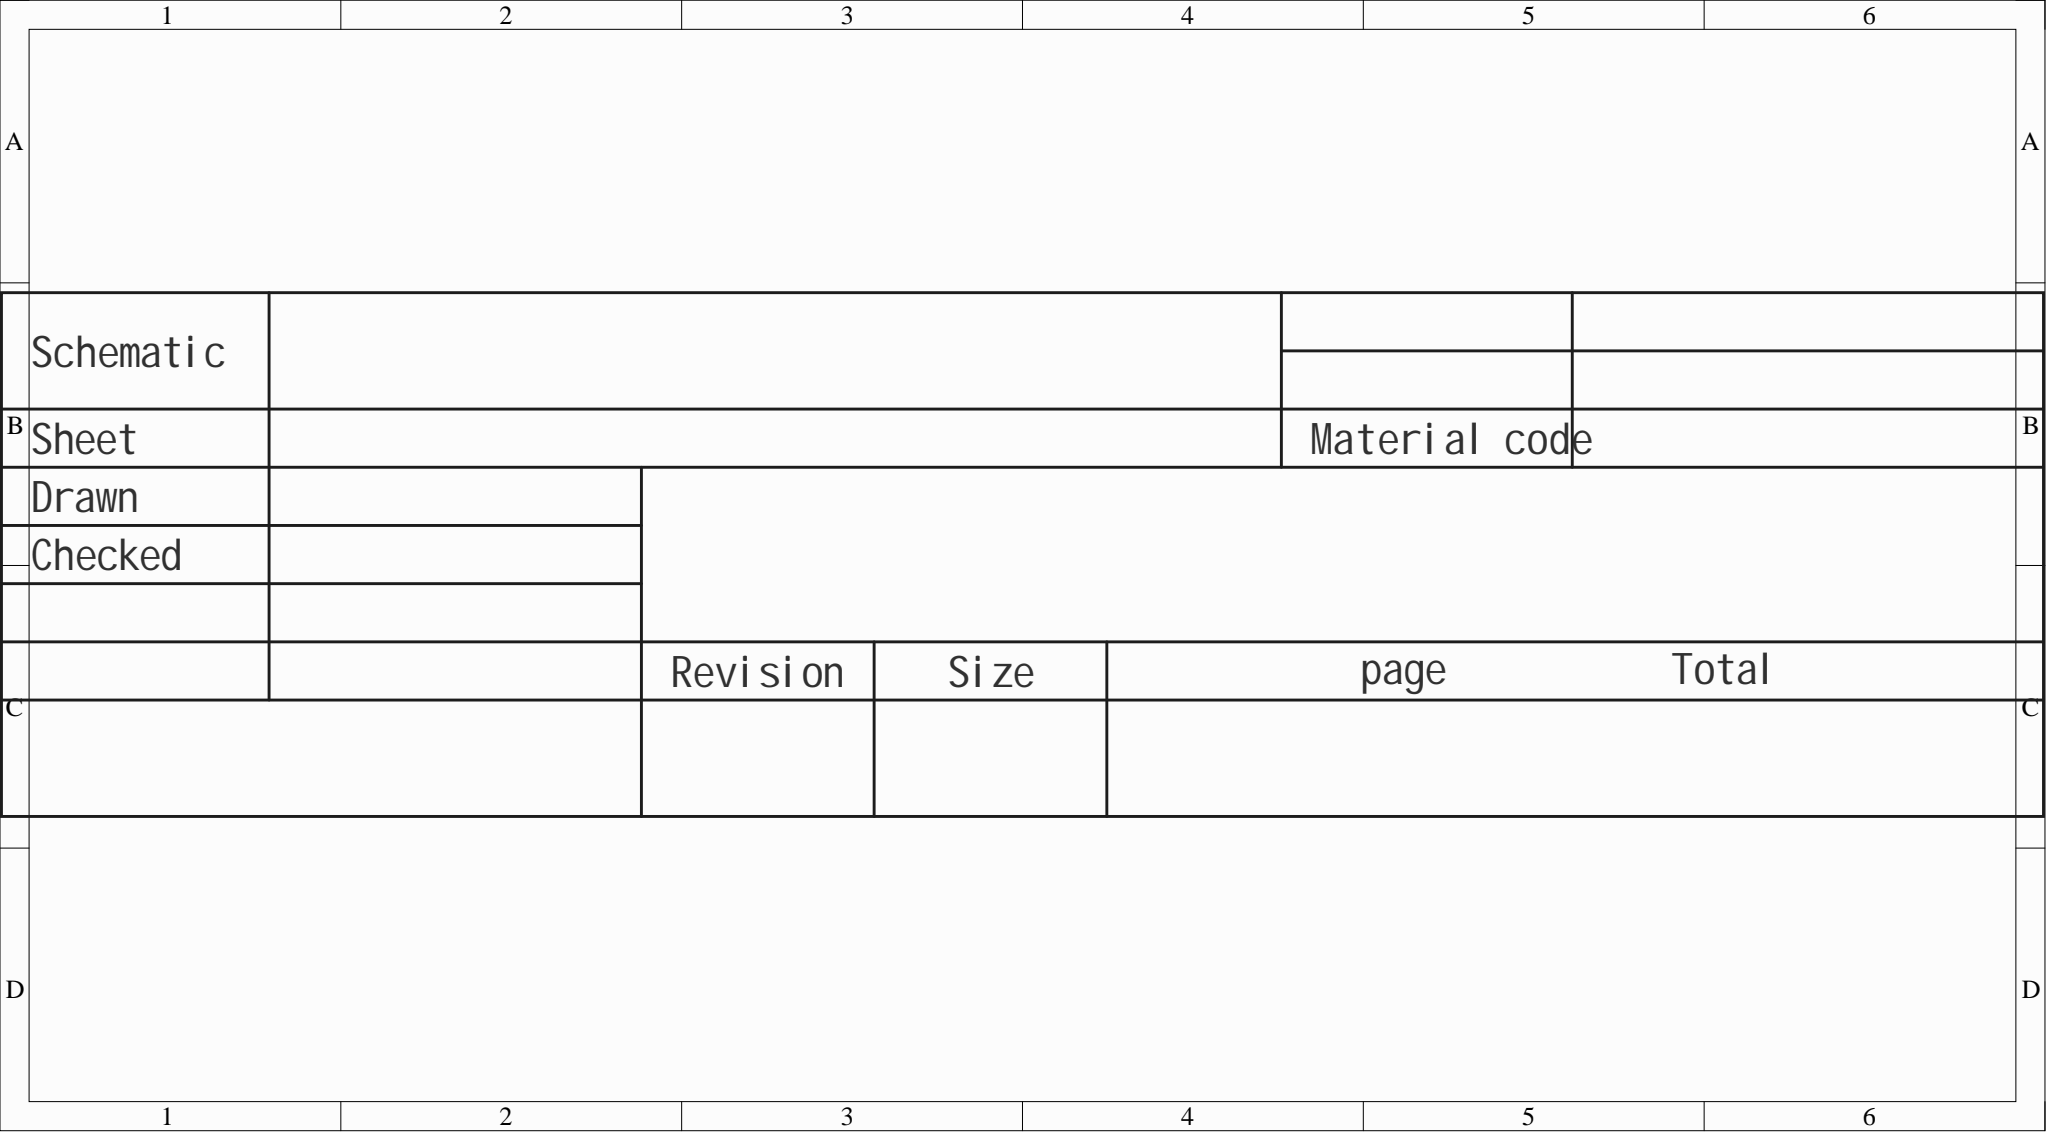Circuit board | Altium Designer | 63 parts | 46 nets
Bill of materials:
Comment,Description,Designator,Footprint,LibRef,Quantity
"100uF","","C1, C2","CAP-TH_BD8.0-P3.50-D0.6-FD_1","100uF","2"
"22uF","Capacitance:22uF;Accuracy:±10%;Rated voltage:16V;ESR:2Ω@100kHz;","C3, C8","CAP-TH_BD5.0-P2.5-D0.5-FD","TAP226K016SCS","2"
"100nF","","C4, C6, C9","CAP-TH_L5.0-W2.5-P5.00-D1.0","100nF","3"
"100UF","Capacitance:100nF;Rated voltage:50V;Ripple current:1A@100kHz;ESR:-;","C5","CAP-TH_BD5.0-P2.00-D0.8-FD","0.1uF 50V 5*11","1"
"4.7uF","Capacitance:4.7uF;Accuracy:±20%;Rated voltage:400V;Ripple current:140mA@100kHz;ESR:23.5Ω@100kHz;","C7","CAP-TH_BD6.3-P2.50-D1.0-FD","LKMC1202G4R7MF","1"
"","","D1","DO_1N4007","D_1N4007A","1"
"","","D2, D3","LED-TH_5mm","LED_TH-R_5mm, LED_TH-G_5mm","2"
"","","H1, H2, H3","HDR-TH_5P-P2.54-V-M","HDR-M_2.54_1x5P","3"
"38K infrared receiver, side-mounted","","OPTO1","OPTO-TH_3P-BD5.9-P2.54","红外38K接收管-侧放","1"
"9013G","","Q1, Q2, Q3, Q4, Q5, Q6, Q7, Q8, Q9, Q10, Q11, Q12, Q13","TO-92-3_L4.9-W3.7-P1.27-L","9013G","13"
"10kΩ","","R1, R7, R13, R15, R18","Res_1/4W","Res_AXIAL-1/4W","5"
"68kΩ","","R2","Res_1/4W","Res_AXIAL-1/4W","1"
"20kΩ","","R3, R23, R25, R30","Res_1/4W","Res_AXIAL-1/4W","4"
"680kΩ","","R4","Res_1/4W","Res_AXIAL-1/4W","1"
"27kΩ","","R5, R24, R28","Res_1/4W","Res_AXIAL-1/4W","3"
"5.1kΩ","","R6, R9, R12, R17, R22","Res_1/4W","Res_AXIAL-1/4W","5"
"51kΩ","","R8, R10, R11, R14, R16, R19, R20","Res_1/4W","Res_AXIAL-1/4W","7"
"100Ω","","R21","Res_1/4W","Res_AXIAL-1/4W","1"
"2kΩ","","R26, R27","Res_1/4W","Res_AXIAL-1/4W","2"
"300Ω","","R29","Res_1/4W","Res_AXIAL-1/4W","1"
"L7805","Fixed output; positive polarity; max input voltage 35V; output voltage 5V; output current 1.2A; ripple rejection (PSRR) 62dB@(120Hz)","U1","TO-220AB-3_L10.4-W4.6-P2.54-L","L7805","1"
"NE555","Single-precision timer 8-PDIP 0 to 70","U2, U4","PDIP-8_L9.6-W6.4-P2.54-LS7.9-BL-1","NE555PE4","2"
"","","U5","DIP-8_L9.9-W6.4-P2.54-LS7.6-BL","语音模块sop-8","1"
Netlist (Protel format):
[
C1
CAP-TH_BD8.0-P3.50-D0.6-FD_1
100uF



]
[
C2
CAP-TH_BD8.0-P3.50-D0.6-FD_1
100uF



]
[
C3
CAP-TH_BD5.0-P2.5-D0.5-FD
22uF



]
[
C4
CAP-TH_L5.0-W2.5-P5.00-D1.0
100nF



]
[
C5
CAP-TH_BD5.0-P2.00-D0.8-FD
100UF



]
[
C6
CAP-TH_L5.0-W2.5-P5.00-D1.0
100nF



]
[
C7
CAP-TH_BD6.3-P2.50-D1.0-FD
4.7uF



]
[
C8
CAP-TH_BD5.0-P2.5-D0.5-FD
22uF



]
[
C9
CAP-TH_L5.0-W2.5-P5.00-D1.0
100nF



]
[
D1
DO_1N4007




]
[
D2
LED-TH_5mm




]
[
D3
LED-TH_5mm




]
[
H1
HDR-TH_5P-P2.54-V-M




]
[
H2
HDR-TH_5P-P2.54-V-M




]
[
H3
HDR-TH_5P-P2.54-V-M




]
[
OPTO1
OPTO-TH_3P-BD5.9-P2.54
38K infrared receiver, side-mounted



]
[
Q1
TO-92-3_L4.9-W3.7-P1.27-L
9013G



]
[
Q2
TO-92-3_L4.9-W3.7-P1.27-L
9013G



]
[
Q3
TO-92-3_L4.9-W3.7-P1.27-L
9013G



]
[
Q4
TO-92-3_L4.9-W3.7-P1.27-L
9013G



]
[
Q5
TO-92-3_L4.9-W3.7-P1.27-L
9013G



]
[
Q6
TO-92-3_L4.9-W3.7-P1.27-L
9013G



]
[
Q7
TO-92-3_L4.9-W3.7-P1.27-L
9013G



]
[
Q8
TO-92-3_L4.9-W3.7-P1.27-L
9013G



]
[
Q9
TO-92-3_L4.9-W3.7-P1.27-L
9013G



]
[
Q10
TO-92-3_L4.9-W3.7-P1.27-L
9013G



]
[
Q11
TO-92-3_L4.9-W3.7-P1.27-L
9013G



]
[
Q12
TO-92-3_L4.9-W3.7-P1.27-L
9013G



]
[
Q13
TO-92-3_L4.9-W3.7-P1.27-L
9013G



]
[
R1
Res_1/4W
10kΩ



]
[
R2
Res_1/4W
68kΩ



]
[
R3
Res_1/4W
20kΩ



]
[
R4
Res_1/4W
680kΩ



]
[
R5
Res_1/4W
27kΩ



]
[
R6
Res_1/4W
5.1kΩ



]
[
R7
Res_1/4W
10kΩ



]
[
R8
Res_1/4W
51kΩ



]
[
R9
Res_1/4W
5.1kΩ



]
[
R10
Res_1/4W
51kΩ



]
[
R11
Res_1/4W
51kΩ



]
[
R12
Res_1/4W
5.1kΩ



]
[
R13
Res_1/4W
10kΩ



]
[
R14
Res_1/4W
51kΩ



]
[
R15
Res_1/4W
10kΩ



]
[
R16
Res_1/4W
51kΩ



]
[
R17
Res_1/4W
5.1kΩ



]
[
R18
Res_1/4W
10kΩ



]
[
R19
Res_1/4W
51kΩ



]
[
R20
Res_1/4W
51kΩ



]
[
R21
Res_1/4W
100Ω



]
[
R22
Res_1/4W
5.1kΩ



]
[
R23
Res_1/4W
20kΩ



]
[
R24
Res_1/4W
27kΩ



]
[
R25
Res_1/4W
20kΩ



]
[
R26
Res_1/4W
2kΩ



]
[
R27
Res_1/4W
2kΩ



]
[
R28
Res_1/4W
27kΩ



]
[
R29
Res_1/4W
300Ω



]
[
R30
Res_1/4W
20kΩ



]
[
U1
TO-220AB-3_L10.4-W4.6-P2.54-L
L7805



]
[
U2
PDIP-8_L9.6-W6.4-P2.54-LS7.9-BL-1
NE555



]
[
U4
PDIP-8_L9.6-W6.4-P2.54-LS7.9-BL-1
NE555



]
[
U5
DIP-8_L9.9-W6.4-P2.54-LS7.6-BL




]
(
OUTD
H1-2
U5-2
)
(
OUTC
H1-1
U5-3
)
(
OUTB
H1-4
R29-1
)
(
OUTA
H1-3
Q12-3
)
(
NetR5_2
R5-2
R6-2
U4-3
)
(
NetR1_1
R1-1
R2-2
U2-7
)
(
NetQ13_3
Q13-3
R29-2
)
(
NetQ13_2
Q13-2
R28-2
)
(
NetQ12_2
Q12-2
R27-2
)
(
NetQ11_2
Q11-2
R26-2
)
(
NetQ9_2
Q9-2
R5-1
)
(
NetQ8_3
Q8-3
Q9-3
Q10-2
R17-2
)
(
NetQ7_3
Q7-3
Q8-2
R16-2
)
(
NetQ6_3
Q6-3
R18-1
)
(
NetQ6_2
Q6-2
R19-1
)
(
NetQ5_3
Q5-3
R15-1
R19-2
R20-2
)
(
NetQ5_2
Q5-2
R14-1
)
(
NetQ4_3
Q4-3
R13-1
R14-2
)
(
NetQ3_3
Q3-3
R12-1
)
(
NetQ3_2
Q3-2
R10-1
)
(
NetQ2_3
Q2-3
R9-1
R11-2
)
(
NetQ1_3
Q1-3
R7-1
R8-2
R10-2
)
(
NetQ1_2
Q1-2
Q11-3
R11-1
)
(
NetOPTO1_3
OPTO1-3
R24-1
)
(
NetOPTO1_1
OPTO1-1
R6-1
)
(
NetD3_2
D3-2
R18-2
)
(
NetD2_2
D2-2
R12-2
)
(
NetD2_1
D2-1
D3-1
U2-3
)
(
NetD1_2
D1-2
R21-1
)
(
NetC9_1
C9-1
U5-1
)
(
NetC8_2
C8-2
R25-1
R26-1
R27-1
R28-1
)
(
NetC8_1
C8-1
Q10-1
R23-1
R24-2
)
(
NetC7_1
C7-1
D1-1
Q7-2
R22-1
)
(
NetC6_1
C6-1
U4-5
)
(
NetC5_1
C5-1
R4-1
U4-6
U4-7
)
(
NetC4_1
C4-1
U2-5
)
(
NetC3_1
C3-1
R2-1
U2-2
U2-6
)
(
K3
H2-3
Q4-2
R20-1
)
(
K2
H2-2
Q2-2
R8-1
)
(
K1
H2-1
R3-1
U4-2
)
(
INC
H1-5
R30-2
U5-7
)
(
INB
H2-4
R22-2
)
(
INA
H3-2
R21-2
)
(
GND
C1-2
C2-2
C3-2
C4-2
C5-2
C6-2
C7-2
C9-2
H2-5
H3-3
H3-5
OPTO1-2
Q1-1
Q2-1
Q3-1
Q4-1
Q5-1
Q6-1
Q7-1
Q8-1
Q9-1
Q11-1
Q12-1
Q13-1
R23-2
R25-2
R30-1
U1-2
U2-1
U4-1
U5-5
)
(
+12V
C1-1
H3-4
Q10-3
R1-2
R3-2
R4-2
R7-2
R9-2
R13-2
R15-2
R16-1
R17-1
U1-1
U2-4
U2-8
U4-4
U4-8
)
(
+5V
C2-1
H3-1
U1-3
U5-4
)